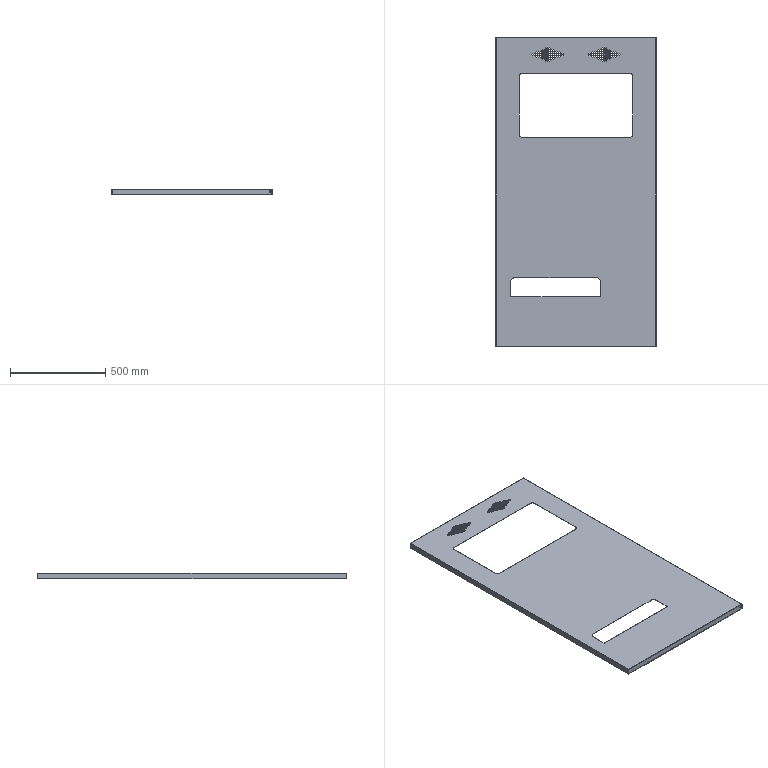Part | SolidWorks | features BaseBody 1 | 1 solid | 838 faces | box 845 x 1628 x 31.2 mm | volume 1603830 mm3 | plane 796 | cylinder 26 | spline 16 | commonest cylinder face diameters 2 x8 4.4 x8 8 x4 30 x4 40 x2